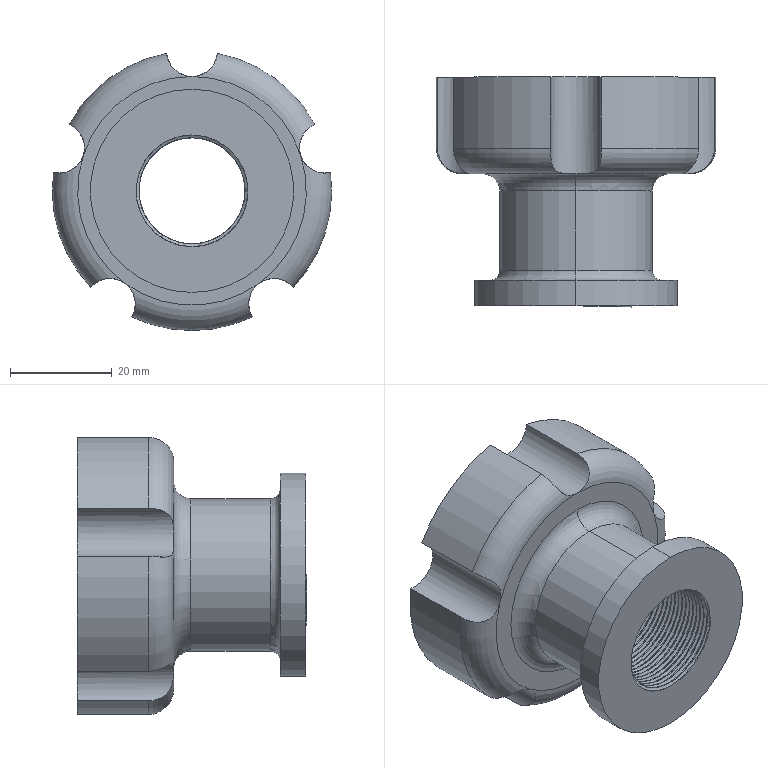Part | SolidWorks | features ICE 1, Revolution 1, SweepThread 1 | 1 solid | 126 faces | box 55 x 45.25 x 54.545 mm | volume 45993 mm3 | cylinder 107 | torus 9 | plane 6 | spline 4 | commonest cylinder face diameters 22 x91 10 x7 55 x5 30 x2 40 x2